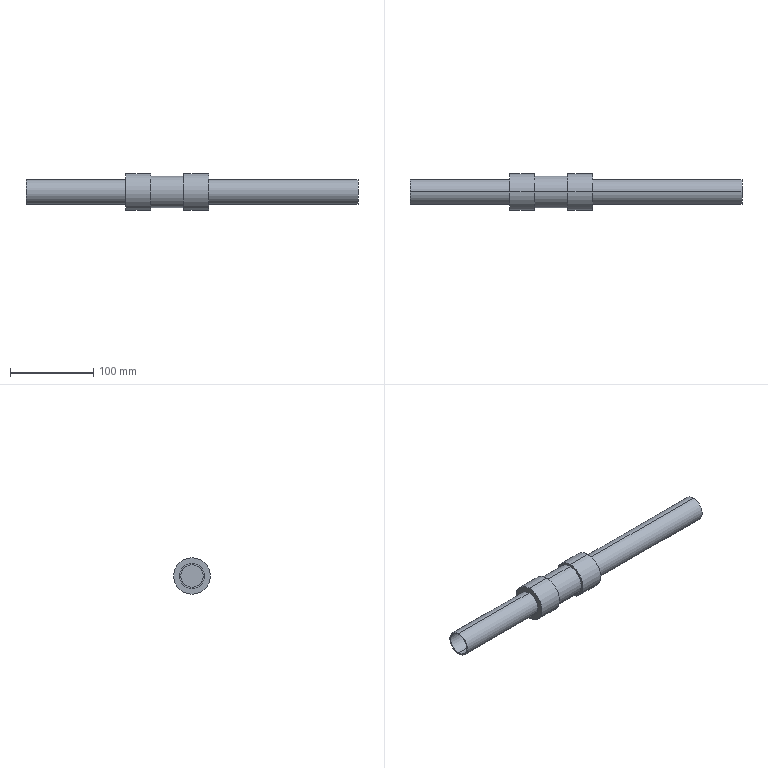Part | SolidWorks | features ICE 1, Revolution 1 | 1 solid | 19 faces | box 400 x 44 x 44 mm | volume 176887 mm3 | cylinder 12 | plane 7 | commonest cylinder face diameters 30 x4 44 x4 27 x2 38 x2
STEP:
#1=CARTESIAN_POINT('',(300.,0.,-13.5));
#2=VERTEX_POINT('',#1);
#3=CARTESIAN_POINT('',(300.,0.,13.5));
#4=VERTEX_POINT('',#3);
#5=CARTESIAN_POINT('',(300.,0.,0.));
#6=DIRECTION('',(-1.,0.,0.));
#7=DIRECTION('',(0.,0.,1.));
#8=AXIS2_PLACEMENT_3D('',#5,#6,#7);
#9=CIRCLE('',#8,13.5);
#10=EDGE_CURVE('',#2,#4,#9,.T.);
#11=ORIENTED_EDGE('',*,*,#10,.F.);
#12=CARTESIAN_POINT('',(0.,0.,-13.5));
#13=VERTEX_POINT('',#12);
#14=CARTESIAN_POINT('',(300.,0.,-13.5));
#15=DIRECTION('',(-1.,0.,0.));
#16=VECTOR('',#15,1000.);
#17=LINE('',#14,#16);
#18=EDGE_CURVE('',#2,#13,#17,.T.);
#19=ORIENTED_EDGE('',*,*,#18,.T.);
#20=CARTESIAN_POINT('',(0.,0.,13.5));
#21=VERTEX_POINT('',#20);
#22=CARTESIAN_POINT('',(0.,0.,0.));
#23=DIRECTION('',(-1.,0.,0.));
#24=DIRECTION('',(0.,0.,1.));
#25=AXIS2_PLACEMENT_3D('',#22,#23,#24);
#26=CIRCLE('',#25,13.5);
#27=EDGE_CURVE('',#13,#21,#26,.T.);
#28=ORIENTED_EDGE('',*,*,#27,.T.);
#29=CARTESIAN_POINT('',(300.,0.,13.5));
#30=DIRECTION('',(-1.,0.,0.));
#31=VECTOR('',#30,1000.);
#32=LINE('',#29,#31);
#33=EDGE_CURVE('',#4,#21,#32,.T.);
#34=ORIENTED_EDGE('',*,*,#33,.F.);
#35=EDGE_LOOP('',(#11,#19,#28,#34));
#36=FACE_OUTER_BOUND('',#35,.T.);
#37=CARTESIAN_POINT('',(300.,0.,0.));
#38=DIRECTION('',(-1.,0.,0.));
#39=DIRECTION('',(0.,0.,1.));
#40=AXIS2_PLACEMENT_3D('',#37,#38,#39);
#41=CYLINDRICAL_SURFACE('',#40,13.5);
#42=ADVANCED_FACE('',(#36),#41,.F.);
#43=CARTESIAN_POINT('',(400.,0.,15.));
#44=VERTEX_POINT('',#43);
#45=CARTESIAN_POINT('',(400.,0.,-15.));
#46=VERTEX_POINT('',#45);
#47=CARTESIAN_POINT('',(400.,0.,0.));
#48=DIRECTION('',(-1.,0.,0.));
#49=DIRECTION('',(0.,0.,1.));
#50=AXIS2_PLACEMENT_3D('',#47,#48,#49);
#51=CIRCLE('',#50,15.);
#52=EDGE_CURVE('',#44,#46,#51,.T.);
#53=ORIENTED_EDGE('',*,*,#52,.T.);
#54=CARTESIAN_POINT('',(220.,0.,-15.));
#55=VERTEX_POINT('',#54);
#56=CARTESIAN_POINT('',(0.,0.,-15.));
#57=DIRECTION('',(-1.,0.,0.));
#58=VECTOR('',#57,1000.);
#59=LINE('',#56,#58);
#60=EDGE_CURVE('',#46,#55,#59,.T.);
#61=ORIENTED_EDGE('',*,*,#60,.T.);
#62=CARTESIAN_POINT('',(220.,0.,15.));
#63=VERTEX_POINT('',#62);
#64=CARTESIAN_POINT('',(220.,0.,0.));
#65=DIRECTION('',(-1.,0.,0.));
#66=DIRECTION('',(0.,0.,1.));
#67=AXIS2_PLACEMENT_3D('',#64,#65,#66);
#68=CIRCLE('',#67,15.);
#69=EDGE_CURVE('',#63,#55,#68,.T.);
#70=ORIENTED_EDGE('',*,*,#69,.F.);
#71=CARTESIAN_POINT('',(0.,0.,15.));
#72=DIRECTION('',(-1.,0.,0.));
#73=VECTOR('',#72,1000.);
#74=LINE('',#71,#73);
#75=EDGE_CURVE('',#44,#63,#74,.T.);
#76=ORIENTED_EDGE('',*,*,#75,.F.);
#77=EDGE_LOOP('',(#53,#61,#70,#76));
#78=FACE_OUTER_BOUND('',#77,.T.);
#79=CARTESIAN_POINT('',(0.,0.,0.));
#80=DIRECTION('',(-1.,0.,0.));
#81=DIRECTION('',(0.,0.,1.));
#82=AXIS2_PLACEMENT_3D('',#79,#80,#81);
#83=CYLINDRICAL_SURFACE('',#82,15.);
#84=ADVANCED_FACE('',(#78),#83,.T.);
#85=CARTESIAN_POINT('',(220.,0.,22.));
#86=VERTEX_POINT('',#85);
#87=CARTESIAN_POINT('',(220.,0.,-22.));
#88=VERTEX_POINT('',#87);
#89=CARTESIAN_POINT('',(220.,0.,0.));
#90=DIRECTION('',(-1.,0.,0.));
#91=DIRECTION('',(0.,0.,1.));
#92=AXIS2_PLACEMENT_3D('',#89,#90,#91);
#93=CIRCLE('',#92,22.);
#94=EDGE_CURVE('',#86,#88,#93,.T.);
#95=ORIENTED_EDGE('',*,*,#94,.T.);
#96=CARTESIAN_POINT('',(190.,0.,-22.));
#97=VERTEX_POINT('',#96);
#98=CARTESIAN_POINT('',(0.,0.,-22.));
#99=DIRECTION('',(-1.,0.,0.));
#100=VECTOR('',#99,1000.);
#101=LINE('',#98,#100);
#102=EDGE_CURVE('',#88,#97,#101,.T.);
#103=ORIENTED_EDGE('',*,*,#102,.T.);
#104=CARTESIAN_POINT('',(190.,0.,22.));
#105=VERTEX_POINT('',#104);
#106=CARTESIAN_POINT('',(190.,0.,0.));
#107=DIRECTION('',(-1.,0.,0.));
#108=DIRECTION('',(0.,0.,1.));
#109=AXIS2_PLACEMENT_3D('',#106,#107,#108);
#110=CIRCLE('',#109,22.);
#111=EDGE_CURVE('',#105,#97,#110,.T.);
#112=ORIENTED_EDGE('',*,*,#111,.F.);
#113=CARTESIAN_POINT('',(0.,0.,22.));
#114=DIRECTION('',(-1.,0.,0.));
#115=VECTOR('',#114,1000.);
#116=LINE('',#113,#115);
#117=EDGE_CURVE('',#86,#105,#116,.T.);
#118=ORIENTED_EDGE('',*,*,#117,.F.);
#119=EDGE_LOOP('',(#95,#103,#112,#118));
#120=FACE_OUTER_BOUND('',#119,.T.);
#121=CARTESIAN_POINT('',(0.,0.,0.));
#122=DIRECTION('',(-1.,0.,0.));
#123=DIRECTION('',(0.,0.,1.));
#124=AXIS2_PLACEMENT_3D('',#121,#122,#123);
#125=CYLINDRICAL_SURFACE('',#124,22.);
#126=ADVANCED_FACE('',(#120),#125,.T.);
#127=CARTESIAN_POINT('',(190.,0.,19.));
#128=VERTEX_POINT('',#127);
#129=CARTESIAN_POINT('',(190.,0.,-19.));
#130=VERTEX_POINT('',#129);
#131=CARTESIAN_POINT('',(190.,0.,0.));
#132=DIRECTION('',(-1.,0.,0.));
#133=DIRECTION('',(0.,0.,1.));
#134=AXIS2_PLACEMENT_3D('',#131,#132,#133);
#135=CIRCLE('',#134,19.);
#136=EDGE_CURVE('',#128,#130,#135,.T.);
#137=ORIENTED_EDGE('',*,*,#136,.T.);
#138=CARTESIAN_POINT('',(150.,0.,-19.));
#139=VERTEX_POINT('',#138);
#140=CARTESIAN_POINT('',(0.,0.,-19.));
#141=DIRECTION('',(-1.,0.,0.));
#142=VECTOR('',#141,1000.);
#143=LINE('',#140,#142);
#144=EDGE_CURVE('',#130,#139,#143,.T.);
#145=ORIENTED_EDGE('',*,*,#144,.T.);
#146=CARTESIAN_POINT('',(150.,0.,19.));
#147=VERTEX_POINT('',#146);
#148=CARTESIAN_POINT('',(150.,0.,0.));
#149=DIRECTION('',(-1.,0.,0.));
#150=DIRECTION('',(0.,0.,1.));
#151=AXIS2_PLACEMENT_3D('',#148,#149,#150);
#152=CIRCLE('',#151,19.);
#153=EDGE_CURVE('',#147,#139,#152,.T.);
#154=ORIENTED_EDGE('',*,*,#153,.F.);
#155=CARTESIAN_POINT('',(0.,0.,19.));
#156=DIRECTION('',(-1.,0.,0.));
#157=VECTOR('',#156,1000.);
#158=LINE('',#155,#157);
#159=EDGE_CURVE('',#128,#147,#158,.T.);
#160=ORIENTED_EDGE('',*,*,#159,.F.);
#161=EDGE_LOOP('',(#137,#145,#154,#160));
#162=FACE_OUTER_BOUND('',#161,.T.);
#163=CARTESIAN_POINT('',(0.,0.,0.));
#164=DIRECTION('',(-1.,0.,0.));
#165=DIRECTION('',(0.,0.,1.));
#166=AXIS2_PLACEMENT_3D('',#163,#164,#165);
#167=CYLINDRICAL_SURFACE('',#166,19.);
#168=ADVANCED_FACE('',(#162),#167,.T.);
#169=CARTESIAN_POINT('',(150.,0.,22.));
#170=VERTEX_POINT('',#169);
#171=CARTESIAN_POINT('',(150.,0.,-22.));
#172=VERTEX_POINT('',#171);
#173=CARTESIAN_POINT('',(150.,0.,0.));
#174=DIRECTION('',(-1.,0.,0.));
#175=DIRECTION('',(0.,0.,1.));
#176=AXIS2_PLACEMENT_3D('',#173,#174,#175);
#177=CIRCLE('',#176,22.);
#178=EDGE_CURVE('',#170,#172,#177,.T.);
#179=ORIENTED_EDGE('',*,*,#178,.T.);
#180=CARTESIAN_POINT('',(120.,0.,-22.));
#181=VERTEX_POINT('',#180);
#182=CARTESIAN_POINT('',(0.,0.,-22.));
#183=DIRECTION('',(-1.,0.,0.));
#184=VECTOR('',#183,1000.);
#185=LINE('',#182,#184);
#186=EDGE_CURVE('',#172,#181,#185,.T.);
#187=ORIENTED_EDGE('',*,*,#186,.T.);
#188=CARTESIAN_POINT('',(120.,0.,22.));
#189=VERTEX_POINT('',#188);
#190=CARTESIAN_POINT('',(120.,0.,0.));
#191=DIRECTION('',(-1.,0.,0.));
#192=DIRECTION('',(0.,0.,1.));
#193=AXIS2_PLACEMENT_3D('',#190,#191,#192);
#194=CIRCLE('',#193,22.);
#195=EDGE_CURVE('',#189,#181,#194,.T.);
#196=ORIENTED_EDGE('',*,*,#195,.F.);
#197=CARTESIAN_POINT('',(0.,0.,22.));
#198=DIRECTION('',(-1.,0.,0.));
#199=VECTOR('',#198,1000.);
#200=LINE('',#197,#199);
#201=EDGE_CURVE('',#170,#189,#200,.T.);
#202=ORIENTED_EDGE('',*,*,#201,.F.);
#203=EDGE_LOOP('',(#179,#187,#196,#202));
#204=FACE_OUTER_BOUND('',#203,.T.);
#205=CARTESIAN_POINT('',(0.,0.,0.));
#206=DIRECTION('',(-1.,0.,0.));
#207=DIRECTION('',(0.,0.,1.));
#208=AXIS2_PLACEMENT_3D('',#205,#206,#207);
#209=CYLINDRICAL_SURFACE('',#208,22.);
#210=ADVANCED_FACE('',(#204),#209,.T.);
#211=CARTESIAN_POINT('',(120.,0.,15.));
#212=VERTEX_POINT('',#211);
#213=CARTESIAN_POINT('',(120.,0.,-15.));
#214=VERTEX_POINT('',#213);
#215=CARTESIAN_POINT('',(120.,0.,0.));
#216=DIRECTION('',(-1.,0.,0.));
#217=DIRECTION('',(0.,0.,1.));
#218=AXIS2_PLACEMENT_3D('',#215,#216,#217);
#219=CIRCLE('',#218,15.);
#220=EDGE_CURVE('',#212,#214,#219,.T.);
#221=ORIENTED_EDGE('',*,*,#220,.T.);
#222=CARTESIAN_POINT('',(0.,0.,-15.));
#223=VERTEX_POINT('',#222);
#224=CARTESIAN_POINT('',(0.,0.,-15.));
#225=DIRECTION('',(-1.,0.,0.));
#226=VECTOR('',#225,1000.);
#227=LINE('',#224,#226);
#228=EDGE_CURVE('',#214,#223,#227,.T.);
#229=ORIENTED_EDGE('',*,*,#228,.T.);
#230=CARTESIAN_POINT('',(0.,0.,15.));
#231=VERTEX_POINT('',#230);
#232=CARTESIAN_POINT('',(0.,0.,0.));
#233=DIRECTION('',(-1.,0.,0.));
#234=DIRECTION('',(0.,0.,1.));
#235=AXIS2_PLACEMENT_3D('',#232,#233,#234);
#236=CIRCLE('',#235,15.);
#237=EDGE_CURVE('',#231,#223,#236,.T.);
#238=ORIENTED_EDGE('',*,*,#237,.F.);
#239=CARTESIAN_POINT('',(0.,0.,15.));
#240=DIRECTION('',(-1.,0.,0.));
#241=VECTOR('',#240,1000.);
#242=LINE('',#239,#241);
#243=EDGE_CURVE('',#212,#231,#242,.T.);
#244=ORIENTED_EDGE('',*,*,#243,.F.);
#245=EDGE_LOOP('',(#221,#229,#238,#244));
#246=FACE_OUTER_BOUND('',#245,.T.);
#247=CARTESIAN_POINT('',(0.,0.,0.));
#248=DIRECTION('',(-1.,0.,0.));
#249=DIRECTION('',(0.,0.,1.));
#250=AXIS2_PLACEMENT_3D('',#247,#248,#249);
#251=CYLINDRICAL_SURFACE('',#250,15.);
#252=ADVANCED_FACE('',(#246),#251,.T.);
#253=CARTESIAN_POINT('',(0.,0.,0.));
#254=DIRECTION('',(-1.,0.,0.));
#255=DIRECTION('',(0.,0.,1.));
#256=AXIS2_PLACEMENT_3D('',#253,#254,#255);
#257=CIRCLE('',#256,13.5);
#258=EDGE_CURVE('',#21,#13,#257,.T.);
#259=ORIENTED_EDGE('',*,*,#258,.F.);
#260=ORIENTED_EDGE('',*,*,#27,.F.);
#261=EDGE_LOOP('',(#259,#260));
#262=FACE_BOUND('',#261,.T.);
#263=ORIENTED_EDGE('',*,*,#237,.T.);
#264=CARTESIAN_POINT('',(0.,0.,0.));
#265=DIRECTION('',(-1.,0.,0.));
#266=DIRECTION('',(0.,0.,1.));
#267=AXIS2_PLACEMENT_3D('',#264,#265,#266);
#268=CIRCLE('',#267,15.);
#269=EDGE_CURVE('',#223,#231,#268,.T.);
#270=ORIENTED_EDGE('',*,*,#269,.T.);
#271=EDGE_LOOP('',(#263,#270));
#272=FACE_OUTER_BOUND('',#271,.T.);
#273=CARTESIAN_POINT('',(0.,0.,0.));
#274=DIRECTION('',(1.,0.,0.));
#275=DIRECTION('',(0.,0.,-1.));
#276=AXIS2_PLACEMENT_3D('',#273,#274,#275);
#277=PLANE('',#276);
#278=ADVANCED_FACE('',(#262,#272),#277,.F.);
#279=ORIENTED_EDGE('',*,*,#228,.F.);
#280=CARTESIAN_POINT('',(120.,0.,0.));
#281=DIRECTION('',(-1.,0.,0.));
#282=DIRECTION('',(0.,0.,1.));
#283=AXIS2_PLACEMENT_3D('',#280,#281,#282);
#284=CIRCLE('',#283,15.);
#285=EDGE_CURVE('',#214,#212,#284,.T.);
#286=ORIENTED_EDGE('',*,*,#285,.T.);
#287=ORIENTED_EDGE('',*,*,#243,.T.);
#288=ORIENTED_EDGE('',*,*,#269,.F.);
#289=EDGE_LOOP('',(#279,#286,#287,#288));
#290=FACE_OUTER_BOUND('',#289,.T.);
#291=CARTESIAN_POINT('',(0.,0.,0.));
#292=DIRECTION('',(-1.,0.,0.));
#293=DIRECTION('',(0.,0.,1.));
#294=AXIS2_PLACEMENT_3D('',#291,#292,#293);
#295=CYLINDRICAL_SURFACE('',#294,15.);
#296=ADVANCED_FACE('',(#290),#295,.T.);
#297=ORIENTED_EDGE('',*,*,#220,.F.);
#298=ORIENTED_EDGE('',*,*,#285,.F.);
#299=EDGE_LOOP('',(#297,#298));
#300=FACE_BOUND('',#299,.T.);
#301=ORIENTED_EDGE('',*,*,#195,.T.);
#302=CARTESIAN_POINT('',(120.,0.,0.));
#303=DIRECTION('',(-1.,0.,0.));
#304=DIRECTION('',(0.,0.,1.));
#305=AXIS2_PLACEMENT_3D('',#302,#303,#304);
#306=CIRCLE('',#305,22.);
#307=EDGE_CURVE('',#181,#189,#306,.T.);
#308=ORIENTED_EDGE('',*,*,#307,.T.);
#309=EDGE_LOOP('',(#301,#308));
#310=FACE_OUTER_BOUND('',#309,.T.);
#311=CARTESIAN_POINT('',(120.,15.,0.));
#312=DIRECTION('',(1.,0.,0.));
#313=DIRECTION('',(0.,0.,-1.));
#314=AXIS2_PLACEMENT_3D('',#311,#312,#313);
#315=PLANE('',#314);
#316=ADVANCED_FACE('',(#300,#310),#315,.F.);
#317=ORIENTED_EDGE('',*,*,#186,.F.);
#318=CARTESIAN_POINT('',(150.,0.,0.));
#319=DIRECTION('',(-1.,0.,0.));
#320=DIRECTION('',(0.,0.,1.));
#321=AXIS2_PLACEMENT_3D('',#318,#319,#320);
#322=CIRCLE('',#321,22.);
#323=EDGE_CURVE('',#172,#170,#322,.T.);
#324=ORIENTED_EDGE('',*,*,#323,.T.);
#325=ORIENTED_EDGE('',*,*,#201,.T.);
#326=ORIENTED_EDGE('',*,*,#307,.F.);
#327=EDGE_LOOP('',(#317,#324,#325,#326));
#328=FACE_OUTER_BOUND('',#327,.T.);
#329=CARTESIAN_POINT('',(0.,0.,0.));
#330=DIRECTION('',(-1.,0.,0.));
#331=DIRECTION('',(0.,0.,1.));
#332=AXIS2_PLACEMENT_3D('',#329,#330,#331);
#333=CYLINDRICAL_SURFACE('',#332,22.);
#334=ADVANCED_FACE('',(#328),#333,.T.);
#335=ORIENTED_EDGE('',*,*,#178,.F.);
#336=ORIENTED_EDGE('',*,*,#323,.F.);
#337=EDGE_LOOP('',(#335,#336));
#338=FACE_OUTER_BOUND('',#337,.T.);
#339=ORIENTED_EDGE('',*,*,#153,.T.);
#340=CARTESIAN_POINT('',(150.,0.,0.));
#341=DIRECTION('',(-1.,0.,0.));
#342=DIRECTION('',(0.,0.,1.));
#343=AXIS2_PLACEMENT_3D('',#340,#341,#342);
#344=CIRCLE('',#343,19.);
#345=EDGE_CURVE('',#139,#147,#344,.T.);
#346=ORIENTED_EDGE('',*,*,#345,.T.);
#347=EDGE_LOOP('',(#339,#346));
#348=FACE_BOUND('',#347,.T.);
#349=CARTESIAN_POINT('',(150.,22.,0.));
#350=DIRECTION('',(-1.,0.,0.));
#351=DIRECTION('',(0.,0.,1.));
#352=AXIS2_PLACEMENT_3D('',#349,#350,#351);
#353=PLANE('',#352);
#354=ADVANCED_FACE('',(#338,#348),#353,.F.);
#355=ORIENTED_EDGE('',*,*,#144,.F.);
#356=CARTESIAN_POINT('',(190.,0.,0.));
#357=DIRECTION('',(-1.,0.,0.));
#358=DIRECTION('',(0.,0.,1.));
#359=AXIS2_PLACEMENT_3D('',#356,#357,#358);
#360=CIRCLE('',#359,19.);
#361=EDGE_CURVE('',#130,#128,#360,.T.);
#362=ORIENTED_EDGE('',*,*,#361,.T.);
#363=ORIENTED_EDGE('',*,*,#159,.T.);
#364=ORIENTED_EDGE('',*,*,#345,.F.);
#365=EDGE_LOOP('',(#355,#362,#363,#364));
#366=FACE_OUTER_BOUND('',#365,.T.);
#367=CARTESIAN_POINT('',(0.,0.,0.));
#368=DIRECTION('',(-1.,0.,0.));
#369=DIRECTION('',(0.,0.,1.));
#370=AXIS2_PLACEMENT_3D('',#367,#368,#369);
#371=CYLINDRICAL_SURFACE('',#370,19.);
#372=ADVANCED_FACE('',(#366),#371,.T.);
#373=ORIENTED_EDGE('',*,*,#136,.F.);
#374=ORIENTED_EDGE('',*,*,#361,.F.);
#375=EDGE_LOOP('',(#373,#374));
#376=FACE_BOUND('',#375,.T.);
#377=ORIENTED_EDGE('',*,*,#111,.T.);
#378=CARTESIAN_POINT('',(190.,0.,0.));
#379=DIRECTION('',(-1.,0.,0.));
#380=DIRECTION('',(0.,0.,1.));
#381=AXIS2_PLACEMENT_3D('',#378,#379,#380);
#382=CIRCLE('',#381,22.);
#383=EDGE_CURVE('',#97,#105,#382,.T.);
#384=ORIENTED_EDGE('',*,*,#383,.T.);
#385=EDGE_LOOP('',(#377,#384));
#386=FACE_OUTER_BOUND('',#385,.T.);
#387=CARTESIAN_POINT('',(190.,19.,0.));
#388=DIRECTION('',(1.,0.,0.));
#389=DIRECTION('',(0.,0.,-1.));
#390=AXIS2_PLACEMENT_3D('',#387,#388,#389);
#391=PLANE('',#390);
#392=ADVANCED_FACE('',(#376,#386),#391,.F.);
#393=ORIENTED_EDGE('',*,*,#102,.F.);
#394=CARTESIAN_POINT('',(220.,0.,0.));
#395=DIRECTION('',(-1.,0.,0.));
#396=DIRECTION('',(0.,0.,1.));
#397=AXIS2_PLACEMENT_3D('',#394,#395,#396);
#398=CIRCLE('',#397,22.);
#399=EDGE_CURVE('',#88,#86,#398,.T.);
#400=ORIENTED_EDGE('',*,*,#399,.T.);
#401=ORIENTED_EDGE('',*,*,#117,.T.);
#402=ORIENTED_EDGE('',*,*,#383,.F.);
#403=EDGE_LOOP('',(#393,#400,#401,#402));
#404=FACE_OUTER_BOUND('',#403,.T.);
#405=CARTESIAN_POINT('',(0.,0.,0.));
#406=DIRECTION('',(-1.,0.,0.));
#407=DIRECTION('',(0.,0.,1.));
#408=AXIS2_PLACEMENT_3D('',#405,#406,#407);
#409=CYLINDRICAL_SURFACE('',#408,22.);
#410=ADVANCED_FACE('',(#404),#409,.T.);
#411=ORIENTED_EDGE('',*,*,#94,.F.);
#412=ORIENTED_EDGE('',*,*,#399,.F.);
#413=EDGE_LOOP('',(#411,#412));
#414=FACE_OUTER_BOUND('',#413,.T.);
#415=ORIENTED_EDGE('',*,*,#69,.T.);
#416=CARTESIAN_POINT('',(220.,0.,0.));
#417=DIRECTION('',(-1.,0.,0.));
#418=DIRECTION('',(0.,0.,1.));
#419=AXIS2_PLACEMENT_3D('',#416,#417,#418);
#420=CIRCLE('',#419,15.);
#421=EDGE_CURVE('',#55,#63,#420,.T.);
#422=ORIENTED_EDGE('',*,*,#421,.T.);
#423=EDGE_LOOP('',(#415,#422));
#424=FACE_BOUND('',#423,.T.);
#425=CARTESIAN_POINT('',(220.,22.,0.));
#426=DIRECTION('',(-1.,0.,0.));
#427=DIRECTION('',(0.,0.,1.));
#428=AXIS2_PLACEMENT_3D('',#425,#426,#427);
#429=PLANE('',#428);
#430=ADVANCED_FACE('',(#414,#424),#429,.F.);
#431=ORIENTED_EDGE('',*,*,#60,.F.);
#432=CARTESIAN_POINT('',(400.,0.,0.));
#433=DIRECTION('',(-1.,0.,0.));
#434=DIRECTION('',(0.,0.,1.));
#435=AXIS2_PLACEMENT_3D('',#432,#433,#434);
#436=CIRCLE('',#435,15.);
#437=EDGE_CURVE('',#46,#44,#436,.T.);
#438=ORIENTED_EDGE('',*,*,#437,.T.);
#439=ORIENTED_EDGE('',*,*,#75,.T.);
#440=ORIENTED_EDGE('',*,*,#421,.F.);
#441=EDGE_LOOP('',(#431,#438,#439,#440));
#442=FACE_OUTER_BOUND('',#441,.T.);
#443=CARTESIAN_POINT('',(0.,0.,0.));
#444=DIRECTION('',(-1.,0.,0.));
#445=DIRECTION('',(0.,0.,1.));
#446=AXIS2_PLACEMENT_3D('',#443,#444,#445);
#447=CYLINDRICAL_SURFACE('',#446,15.);
#448=ADVANCED_FACE('',(#442),#447,.T.);
#449=ORIENTED_EDGE('',*,*,#52,.F.);
#450=ORIENTED_EDGE('',*,*,#437,.F.);
#451=EDGE_LOOP('',(#449,#450));
#452=FACE_OUTER_BOUND('',#451,.T.);
#453=CARTESIAN_POINT('',(400.,15.,0.));
#454=DIRECTION('',(-1.,0.,0.));
#455=DIRECTION('',(0.,0.,1.));
#456=AXIS2_PLACEMENT_3D('',#453,#454,#455);
#457=PLANE('',#456);
#458=ADVANCED_FACE('',(#452),#457,.F.);
#459=ORIENTED_EDGE('',*,*,#18,.F.);
#460=CARTESIAN_POINT('',(300.,0.,0.));
#461=DIRECTION('',(-1.,0.,0.));
#462=DIRECTION('',(0.,0.,1.));
#463=AXIS2_PLACEMENT_3D('',#460,#461,#462);
#464=CIRCLE('',#463,13.5);
#465=EDGE_CURVE('',#4,#2,#464,.T.);
#466=ORIENTED_EDGE('',*,*,#465,.F.);
#467=ORIENTED_EDGE('',*,*,#33,.T.);
#468=ORIENTED_EDGE('',*,*,#258,.T.);
#469=EDGE_LOOP('',(#459,#466,#467,#468));
#470=FACE_OUTER_BOUND('',#469,.T.);
#471=CARTESIAN_POINT('',(300.,0.,0.));
#472=DIRECTION('',(-1.,0.,0.));
#473=DIRECTION('',(0.,0.,1.));
#474=AXIS2_PLACEMENT_3D('',#471,#472,#473);
#475=CYLINDRICAL_SURFACE('',#474,13.5);
#476=ADVANCED_FACE('',(#470),#475,.F.);
#477=ORIENTED_EDGE('',*,*,#465,.T.);
#478=ORIENTED_EDGE('',*,*,#10,.T.);
#479=EDGE_LOOP('',(#477,#478));
#480=FACE_OUTER_BOUND('',#479,.T.);
#481=CARTESIAN_POINT('',(300.,0.,0.));
#482=DIRECTION('',(-1.,0.,0.));
#483=DIRECTION('',(0.,0.,1.));
#484=AXIS2_PLACEMENT_3D('',#481,#482,#483);
#485=PLANE('',#484);
#486=ADVANCED_FACE('',(#480),#485,.T.);
#487=CLOSED_SHELL('',(#42,#84,#126,#168,#210,#252,#278,#296,#316,#334,#354,#372,#392,#410,#430,#448,#458,#476,#486));
#488=MANIFOLD_SOLID_BREP('',#487);
#489=CARTESIAN_POINT('',(0.,0.,0.));
#490=DIRECTION('',(0.,0.,1.));
#491=DIRECTION('',(1.,0.,0.));
#492=AXIS2_PLACEMENT_3D('',#489,#490,#491);
#493=(LENGTH_UNIT()NAMED_UNIT(*)SI_UNIT(.MILLI.,.METRE.));
#494=UNCERTAINTY_MEASURE_WITH_UNIT(LENGTH_MEASURE(0.00001),#493,'','');
#495=(NAMED_UNIT(*)PLANE_ANGLE_UNIT()SI_UNIT($,.RADIAN.));
#496=(NAMED_UNIT(*)SI_UNIT($,.STERADIAN.)SOLID_ANGLE_UNIT());
#497=(GEOMETRIC_REPRESENTATION_CONTEXT(3)GLOBAL_UNCERTAINTY_ASSIGNED_CONTEXT((#494))GLOBAL_UNIT_ASSIGNED_CONTEXT((#493,#495,#496))REPRESENTATION_CONTEXT('',''));
#498=ADVANCED_BREP_SHAPE_REPRESENTATION('',(#488,#492),#497);